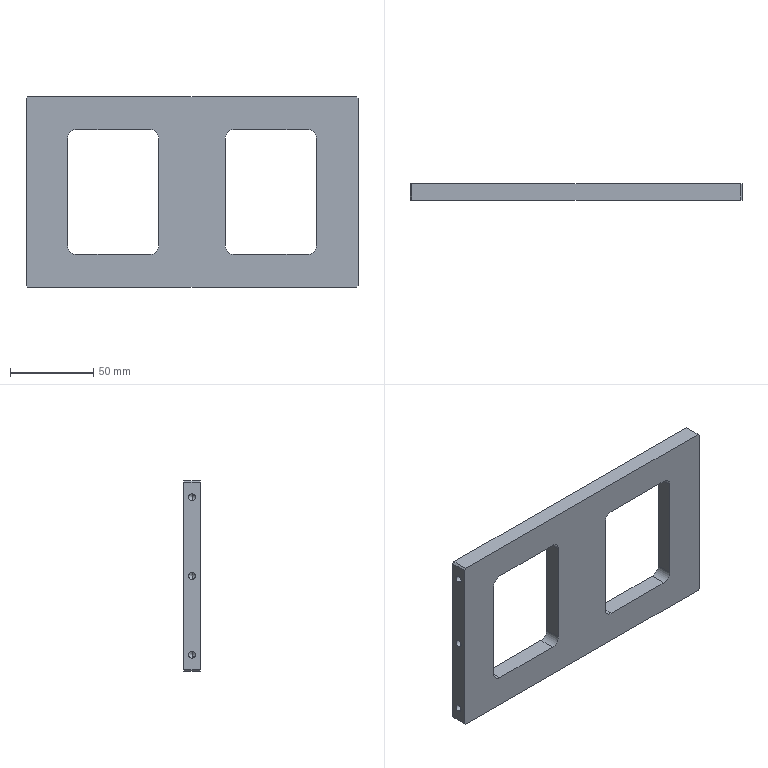Part | SolidWorks | features BaseBody 1 | 1 solid | 50 faces | box 200 x 10 x 115 mm | volume 146843 mm3 | cylinder 20 | plane 18 | cone 12 | commonest cylinder face diameters 4.2 x12 10 x8
STEP:
#1=CARTESIAN_POINT('',(87.6,0.,-45.4));
#2=VERTEX_POINT('',#1);
#3=CARTESIAN_POINT('',(100.,0.,-45.4));
#4=VERTEX_POINT('',#3);
#5=CARTESIAN_POINT('',(100.,0.,-45.4));
#6=DIRECTION('',(1.,0.,0.));
#7=VECTOR('',#6,1000.);
#8=LINE('',#5,#7);
#9=EDGE_CURVE('',#2,#4,#8,.T.);
#10=ORIENTED_EDGE('',*,*,#9,.F.);
#11=CARTESIAN_POINT('',(87.6,0.,-49.6));
#12=VERTEX_POINT('',#11);
#13=CARTESIAN_POINT('',(87.6,0.,-47.5));
#14=DIRECTION('',(1.,0.,0.));
#15=DIRECTION('',(0.,0.,-1.));
#16=AXIS2_PLACEMENT_3D('',#13,#14,#15);
#17=CIRCLE('',#16,2.1);
#18=EDGE_CURVE('',#12,#2,#17,.T.);
#19=ORIENTED_EDGE('',*,*,#18,.F.);
#20=CARTESIAN_POINT('',(100.,0.,-49.6));
#21=VERTEX_POINT('',#20);
#22=CARTESIAN_POINT('',(100.,0.,-49.6));
#23=DIRECTION('',(1.,0.,0.));
#24=VECTOR('',#23,1000.);
#25=LINE('',#22,#24);
#26=EDGE_CURVE('',#12,#21,#25,.T.);
#27=ORIENTED_EDGE('',*,*,#26,.T.);
#28=CARTESIAN_POINT('',(100.,0.,-47.5));
#29=DIRECTION('',(1.,0.,0.));
#30=DIRECTION('',(0.,0.,-1.));
#31=AXIS2_PLACEMENT_3D('',#28,#29,#30);
#32=CIRCLE('',#31,2.1);
#33=EDGE_CURVE('',#21,#4,#32,.T.);
#34=ORIENTED_EDGE('',*,*,#33,.T.);
#35=EDGE_LOOP('',(#10,#19,#27,#34));
#36=FACE_OUTER_BOUND('',#35,.T.);
#37=CARTESIAN_POINT('',(100.,0.,-47.5));
#38=DIRECTION('',(1.,0.,0.));
#39=DIRECTION('',(0.,0.,-1.));
#40=AXIS2_PLACEMENT_3D('',#37,#38,#39);
#41=CYLINDRICAL_SURFACE('',#40,2.1);
#42=ADVANCED_FACE('',(#36),#41,.F.);
#43=CARTESIAN_POINT('',(86.338,0.,-47.5));
#44=VERTEX_POINT('',#43);
#45=CARTESIAN_POINT('',(87.6,0.,-45.4));
#46=DIRECTION('',(0.515,0.,0.8572));
#47=VECTOR('',#46,1000.);
#48=LINE('',#45,#47);
#49=EDGE_CURVE('',#44,#2,#48,.T.);
#50=ORIENTED_EDGE('',*,*,#49,.F.);
#51=CARTESIAN_POINT('',(87.6,0.,-49.6));
#52=DIRECTION('',(0.515,0.,-0.8572));
#53=VECTOR('',#52,1000.);
#54=LINE('',#51,#53);
#55=EDGE_CURVE('',#44,#12,#54,.T.);
#56=ORIENTED_EDGE('',*,*,#55,.T.);
#57=ORIENTED_EDGE('',*,*,#18,.T.);
#58=EDGE_LOOP('',(#50,#56,#57));
#59=FACE_OUTER_BOUND('',#58,.T.);
#60=CARTESIAN_POINT('',(87.6,0.,-47.5));
#61=DIRECTION('',(1.,0.,0.));
#62=DIRECTION('',(0.,0.,-1.));
#63=AXIS2_PLACEMENT_3D('',#60,#61,#62);
#64=CONICAL_SURFACE('',#63,2.1,1.03);
#65=ADVANCED_FACE('',(#59),#64,.F.);
#66=CARTESIAN_POINT('',(87.6,0.,2.1));
#67=VERTEX_POINT('',#66);
#68=CARTESIAN_POINT('',(100.,0.,2.1));
#69=VERTEX_POINT('',#68);
#70=CARTESIAN_POINT('',(100.,0.,2.1));
#71=DIRECTION('',(1.,0.,0.));
#72=VECTOR('',#71,1000.);
#73=LINE('',#70,#72);
#74=EDGE_CURVE('',#67,#69,#73,.T.);
#75=ORIENTED_EDGE('',*,*,#74,.F.);
#76=CARTESIAN_POINT('',(87.6,0.,-2.1));
#77=VERTEX_POINT('',#76);
#78=CARTESIAN_POINT('',(87.6,0.,0.));
#79=DIRECTION('',(1.,0.,0.));
#80=DIRECTION('',(0.,0.,-1.));
#81=AXIS2_PLACEMENT_3D('',#78,#79,#80);
#82=CIRCLE('',#81,2.1);
#83=EDGE_CURVE('',#77,#67,#82,.T.);
#84=ORIENTED_EDGE('',*,*,#83,.F.);
#85=CARTESIAN_POINT('',(100.,0.,-2.1));
#86=VERTEX_POINT('',#85);
#87=CARTESIAN_POINT('',(100.,0.,-2.1));
#88=DIRECTION('',(1.,0.,0.));
#89=VECTOR('',#88,1000.);
#90=LINE('',#87,#89);
#91=EDGE_CURVE('',#77,#86,#90,.T.);
#92=ORIENTED_EDGE('',*,*,#91,.T.);
#93=CARTESIAN_POINT('',(100.,0.,0.));
#94=DIRECTION('',(1.,0.,0.));
#95=DIRECTION('',(0.,0.,-1.));
#96=AXIS2_PLACEMENT_3D('',#93,#94,#95);
#97=CIRCLE('',#96,2.1);
#98=EDGE_CURVE('',#86,#69,#97,.T.);
#99=ORIENTED_EDGE('',*,*,#98,.T.);
#100=EDGE_LOOP('',(#75,#84,#92,#99));
#101=FACE_OUTER_BOUND('',#100,.T.);
#102=CARTESIAN_POINT('',(100.,0.,0.));
#103=DIRECTION('',(1.,0.,0.));
#104=DIRECTION('',(0.,0.,-1.));
#105=AXIS2_PLACEMENT_3D('',#102,#103,#104);
#106=CYLINDRICAL_SURFACE('',#105,2.1);
#107=ADVANCED_FACE('',(#101),#106,.F.);
#108=CARTESIAN_POINT('',(86.338,0.,0.));
#109=VERTEX_POINT('',#108);
#110=CARTESIAN_POINT('',(87.6,0.,2.1));
#111=DIRECTION('',(0.515,0.,0.8572));
#112=VECTOR('',#111,1000.);
#113=LINE('',#110,#112);
#114=EDGE_CURVE('',#109,#67,#113,.T.);
#115=ORIENTED_EDGE('',*,*,#114,.F.);
#116=CARTESIAN_POINT('',(87.6,0.,-2.1));
#117=DIRECTION('',(0.515,0.,-0.8572));
#118=VECTOR('',#117,1000.);
#119=LINE('',#116,#118);
#120=EDGE_CURVE('',#109,#77,#119,.T.);
#121=ORIENTED_EDGE('',*,*,#120,.T.);
#122=ORIENTED_EDGE('',*,*,#83,.T.);
#123=EDGE_LOOP('',(#115,#121,#122));
#124=FACE_OUTER_BOUND('',#123,.T.);
#125=CARTESIAN_POINT('',(87.6,0.,0.));
#126=DIRECTION('',(1.,0.,0.));
#127=DIRECTION('',(0.,0.,-1.));
#128=AXIS2_PLACEMENT_3D('',#125,#126,#127);
#129=CONICAL_SURFACE('',#128,2.1,1.03);
#130=ADVANCED_FACE('',(#124),#129,.F.);
#131=CARTESIAN_POINT('',(87.6,0.,49.6));
#132=VERTEX_POINT('',#131);
#133=CARTESIAN_POINT('',(100.,0.,49.6));
#134=VERTEX_POINT('',#133);
#135=CARTESIAN_POINT('',(100.,0.,49.6));
#136=DIRECTION('',(1.,0.,0.));
#137=VECTOR('',#136,1000.);
#138=LINE('',#135,#137);
#139=EDGE_CURVE('',#132,#134,#138,.T.);
#140=ORIENTED_EDGE('',*,*,#139,.F.);
#141=CARTESIAN_POINT('',(87.6,0.,45.4));
#142=VERTEX_POINT('',#141);
#143=CARTESIAN_POINT('',(87.6,0.,47.5));
#144=DIRECTION('',(1.,0.,0.));
#145=DIRECTION('',(0.,0.,-1.));
#146=AXIS2_PLACEMENT_3D('',#143,#144,#145);
#147=CIRCLE('',#146,2.1);
#148=EDGE_CURVE('',#142,#132,#147,.T.);
#149=ORIENTED_EDGE('',*,*,#148,.F.);
#150=CARTESIAN_POINT('',(100.,0.,45.4));
#151=VERTEX_POINT('',#150);
#152=CARTESIAN_POINT('',(100.,0.,45.4));
#153=DIRECTION('',(1.,0.,0.));
#154=VECTOR('',#153,1000.);
#155=LINE('',#152,#154);
#156=EDGE_CURVE('',#142,#151,#155,.T.);
#157=ORIENTED_EDGE('',*,*,#156,.T.);
#158=CARTESIAN_POINT('',(100.,0.,47.5));
#159=DIRECTION('',(1.,0.,0.));
#160=DIRECTION('',(0.,0.,-1.));
#161=AXIS2_PLACEMENT_3D('',#158,#159,#160);
#162=CIRCLE('',#161,2.1);
#163=EDGE_CURVE('',#151,#134,#162,.T.);
#164=ORIENTED_EDGE('',*,*,#163,.T.);
#165=EDGE_LOOP('',(#140,#149,#157,#164));
#166=FACE_OUTER_BOUND('',#165,.T.);
#167=CARTESIAN_POINT('',(100.,0.,47.5));
#168=DIRECTION('',(1.,0.,0.));
#169=DIRECTION('',(0.,0.,-1.));
#170=AXIS2_PLACEMENT_3D('',#167,#168,#169);
#171=CYLINDRICAL_SURFACE('',#170,2.1);
#172=ADVANCED_FACE('',(#166),#171,.F.);
#173=CARTESIAN_POINT('',(86.338,0.,47.5));
#174=VERTEX_POINT('',#173);
#175=CARTESIAN_POINT('',(87.6,0.,49.6));
#176=DIRECTION('',(0.515,0.,0.8572));
#177=VECTOR('',#176,1000.);
#178=LINE('',#175,#177);
#179=EDGE_CURVE('',#174,#132,#178,.T.);
#180=ORIENTED_EDGE('',*,*,#179,.F.);
#181=CARTESIAN_POINT('',(87.6,0.,45.4));
#182=DIRECTION('',(0.515,0.,-0.8572));
#183=VECTOR('',#182,1000.);
#184=LINE('',#181,#183);
#185=EDGE_CURVE('',#174,#142,#184,.T.);
#186=ORIENTED_EDGE('',*,*,#185,.T.);
#187=ORIENTED_EDGE('',*,*,#148,.T.);
#188=EDGE_LOOP('',(#180,#186,#187));
#189=FACE_OUTER_BOUND('',#188,.T.);
#190=CARTESIAN_POINT('',(87.6,0.,47.5));
#191=DIRECTION('',(1.,0.,0.));
#192=DIRECTION('',(0.,0.,-1.));
#193=AXIS2_PLACEMENT_3D('',#190,#191,#192);
#194=CONICAL_SURFACE('',#193,2.1,1.03);
#195=ADVANCED_FACE('',(#189),#194,.F.);
#196=CARTESIAN_POINT('',(75.,-5.,-32.5));
#197=VERTEX_POINT('',#196);
#198=CARTESIAN_POINT('',(75.,5.,-32.5));
#199=VERTEX_POINT('',#198);
#200=CARTESIAN_POINT('',(75.,-98.005,-32.5));
#201=DIRECTION('',(0.,1.,0.));
#202=VECTOR('',#201,1000.);
#203=LINE('',#200,#202);
#204=EDGE_CURVE('',#197,#199,#203,.T.);
#205=ORIENTED_EDGE('',*,*,#204,.T.);
#206=CARTESIAN_POINT('',(70.,5.,-37.5));
#207=VERTEX_POINT('',#206);
#208=CARTESIAN_POINT('',(70.,5.,-32.5));
#209=DIRECTION('',(0.,1.,0.));
#210=DIRECTION('',(0.,0.,-1.));
#211=AXIS2_PLACEMENT_3D('',#208,#209,#210);
#212=CIRCLE('',#211,5.);
#213=EDGE_CURVE('',#199,#207,#212,.T.);
#214=ORIENTED_EDGE('',*,*,#213,.T.);
#215=CARTESIAN_POINT('',(70.,-5.,-37.5));
#216=VERTEX_POINT('',#215);
#217=CARTESIAN_POINT('',(70.,-98.005,-37.5));
#218=DIRECTION('',(0.,1.,0.));
#219=VECTOR('',#218,1000.);
#220=LINE('',#217,#219);
#221=EDGE_CURVE('',#216,#207,#220,.T.);
#222=ORIENTED_EDGE('',*,*,#221,.F.);
#223=CARTESIAN_POINT('',(70.,-5.,-32.5));
#224=DIRECTION('',(0.,1.,0.));
#225=DIRECTION('',(0.,0.,-1.));
#226=AXIS2_PLACEMENT_3D('',#223,#224,#225);
#227=CIRCLE('',#226,5.);
#228=EDGE_CURVE('',#197,#216,#227,.T.);
#229=ORIENTED_EDGE('',*,*,#228,.F.);
#230=EDGE_LOOP('',(#205,#214,#222,#229));
#231=FACE_OUTER_BOUND('',#230,.T.);
#232=CARTESIAN_POINT('',(70.,-98.005,-32.5));
#233=DIRECTION('',(0.,1.,0.));
#234=DIRECTION('',(0.,0.,1.));
#235=AXIS2_PLACEMENT_3D('',#232,#233,#234);
#236=CYLINDRICAL_SURFACE('',#235,5.);
#237=ADVANCED_FACE('',(#231),#236,.F.);
#238=CARTESIAN_POINT('',(75.,-5.,32.5));
#239=VERTEX_POINT('',#238);
#240=CARTESIAN_POINT('',(75.,5.,32.5));
#241=VERTEX_POINT('',#240);
#242=CARTESIAN_POINT('',(75.,-98.005,32.5));
#243=DIRECTION('',(0.,1.,0.));
#244=VECTOR('',#243,1000.);
#245=LINE('',#242,#244);
#246=EDGE_CURVE('',#239,#241,#245,.T.);
#247=ORIENTED_EDGE('',*,*,#246,.T.);
#248=CARTESIAN_POINT('',(75.,5.,-32.5));
#249=DIRECTION('',(0.,0.,-1.));
#250=VECTOR('',#249,1000.);
#251=LINE('',#248,#250);
#252=EDGE_CURVE('',#241,#199,#251,.T.);
#253=ORIENTED_EDGE('',*,*,#252,.T.);
#254=ORIENTED_EDGE('',*,*,#204,.F.);
#255=CARTESIAN_POINT('',(75.,-5.,-32.5));
#256=DIRECTION('',(0.,0.,-1.));
#257=VECTOR('',#256,1000.);
#258=LINE('',#255,#257);
#259=EDGE_CURVE('',#239,#197,#258,.T.);
#260=ORIENTED_EDGE('',*,*,#259,.F.);
#261=EDGE_LOOP('',(#247,#253,#254,#260));
#262=FACE_OUTER_BOUND('',#261,.T.);
#263=CARTESIAN_POINT('',(75.,-98.005,-32.5));
#264=DIRECTION('',(1.,0.,0.));
#265=DIRECTION('',(0.,1.,0.));
#266=AXIS2_PLACEMENT_3D('',#263,#264,#265);
#267=PLANE('',#266);
#268=ADVANCED_FACE('',(#262),#267,.F.);
#269=CARTESIAN_POINT('',(70.,-5.,37.5));
#270=VERTEX_POINT('',#269);
#271=CARTESIAN_POINT('',(70.,5.,37.5));
#272=VERTEX_POINT('',#271);
#273=CARTESIAN_POINT('',(70.,-98.005,37.5));
#274=DIRECTION('',(0.,1.,0.));
#275=VECTOR('',#274,1000.);
#276=LINE('',#273,#275);
#277=EDGE_CURVE('',#270,#272,#276,.T.);
#278=ORIENTED_EDGE('',*,*,#277,.T.);
#279=CARTESIAN_POINT('',(70.,5.,32.5));
#280=DIRECTION('',(0.,1.,0.));
#281=DIRECTION('',(0.,0.,1.));
#282=AXIS2_PLACEMENT_3D('',#279,#280,#281);
#283=CIRCLE('',#282,5.);
#284=EDGE_CURVE('',#272,#241,#283,.T.);
#285=ORIENTED_EDGE('',*,*,#284,.T.);
#286=ORIENTED_EDGE('',*,*,#246,.F.);
#287=CARTESIAN_POINT('',(70.,-5.,32.5));
#288=DIRECTION('',(0.,1.,0.));
#289=DIRECTION('',(0.,0.,-1.));
#290=AXIS2_PLACEMENT_3D('',#287,#288,#289);
#291=CIRCLE('',#290,5.);
#292=EDGE_CURVE('',#270,#239,#291,.T.);
#293=ORIENTED_EDGE('',*,*,#292,.F.);
#294=EDGE_LOOP('',(#278,#285,#286,#293));
#295=FACE_OUTER_BOUND('',#294,.T.);
#296=CARTESIAN_POINT('',(70.,-98.005,32.5));
#297=DIRECTION('',(0.,1.,0.));
#298=DIRECTION('',(0.,0.,1.));
#299=AXIS2_PLACEMENT_3D('',#296,#297,#298);
#300=CYLINDRICAL_SURFACE('',#299,5.);
#301=ADVANCED_FACE('',(#295),#300,.F.);
#302=CARTESIAN_POINT('',(25.,-5.,37.5));
#303=VERTEX_POINT('',#302);
#304=CARTESIAN_POINT('',(25.,5.,37.5));
#305=VERTEX_POINT('',#304);
#306=CARTESIAN_POINT('',(25.,-98.005,37.5));
#307=DIRECTION('',(0.,1.,0.));
#308=VECTOR('',#307,1000.);
#309=LINE('',#306,#308);
#310=EDGE_CURVE('',#303,#305,#309,.T.);
#311=ORIENTED_EDGE('',*,*,#310,.T.);
#312=CARTESIAN_POINT('',(25.,5.,37.5));
#313=DIRECTION('',(1.,0.,0.));
#314=VECTOR('',#313,1000.);
#315=LINE('',#312,#314);
#316=EDGE_CURVE('',#305,#272,#315,.T.);
#317=ORIENTED_EDGE('',*,*,#316,.T.);
#318=ORIENTED_EDGE('',*,*,#277,.F.);
#319=CARTESIAN_POINT('',(25.,-5.,37.5));
#320=DIRECTION('',(1.,0.,0.));
#321=VECTOR('',#320,1000.);
#322=LINE('',#319,#321);
#323=EDGE_CURVE('',#303,#270,#322,.T.);
#324=ORIENTED_EDGE('',*,*,#323,.F.);
#325=EDGE_LOOP('',(#311,#317,#318,#324));
#326=FACE_OUTER_BOUND('',#325,.T.);
#327=CARTESIAN_POINT('',(25.,-98.005,37.5));
#328=DIRECTION('',(0.,0.,1.));
#329=DIRECTION('',(1.,0.,0.));
#330=AXIS2_PLACEMENT_3D('',#327,#328,#329);
#331=PLANE('',#330);
#332=ADVANCED_FACE('',(#326),#331,.F.);
#333=CARTESIAN_POINT('',(20.,-5.,32.5));
#334=VERTEX_POINT('',#333);
#335=CARTESIAN_POINT('',(20.,5.,32.5));
#336=VERTEX_POINT('',#335);
#337=CARTESIAN_POINT('',(20.,-98.005,32.5));
#338=DIRECTION('',(0.,1.,0.));
#339=VECTOR('',#338,1000.);
#340=LINE('',#337,#339);
#341=EDGE_CURVE('',#334,#336,#340,.T.);
#342=ORIENTED_EDGE('',*,*,#341,.T.);
#343=CARTESIAN_POINT('',(25.,5.,32.5));
#344=DIRECTION('',(0.,1.,0.));
#345=DIRECTION('',(0.,0.,1.));
#346=AXIS2_PLACEMENT_3D('',#343,#344,#345);
#347=CIRCLE('',#346,5.);
#348=EDGE_CURVE('',#336,#305,#347,.T.);
#349=ORIENTED_EDGE('',*,*,#348,.T.);
#350=ORIENTED_EDGE('',*,*,#310,.F.);
#351=CARTESIAN_POINT('',(25.,-5.,32.5));
#352=DIRECTION('',(0.,1.,0.));
#353=DIRECTION('',(0.,0.,-1.));
#354=AXIS2_PLACEMENT_3D('',#351,#352,#353);
#355=CIRCLE('',#354,5.);
#356=EDGE_CURVE('',#334,#303,#355,.T.);
#357=ORIENTED_EDGE('',*,*,#356,.F.);
#358=EDGE_LOOP('',(#342,#349,#350,#357));
#359=FACE_OUTER_BOUND('',#358,.T.);
#360=CARTESIAN_POINT('',(25.,-98.005,32.5));
#361=DIRECTION('',(0.,1.,0.));
#362=DIRECTION('',(0.,0.,1.));
#363=AXIS2_PLACEMENT_3D('',#360,#361,#362);
#364=CYLINDRICAL_SURFACE('',#363,5.);
#365=ADVANCED_FACE('',(#359),#364,.F.);
#366=CARTESIAN_POINT('',(20.,-5.,-32.5));
#367=VERTEX_POINT('',#366);
#368=CARTESIAN_POINT('',(20.,5.,-32.5));
#369=VERTEX_POINT('',#368);
#370=CARTESIAN_POINT('',(20.,-98.005,-32.5));
#371=DIRECTION('',(0.,1.,0.));
#372=VECTOR('',#371,1000.);
#373=LINE('',#370,#372);
#374=EDGE_CURVE('',#367,#369,#373,.T.);
#375=ORIENTED_EDGE('',*,*,#374,.T.);
#376=CARTESIAN_POINT('',(20.,5.,-32.5));
#377=DIRECTION('',(0.,0.,1.));
#378=VECTOR('',#377,1000.);
#379=LINE('',#376,#378);
#380=EDGE_CURVE('',#369,#336,#379,.T.);
#381=ORIENTED_EDGE('',*,*,#380,.T.);
#382=ORIENTED_EDGE('',*,*,#341,.F.);
#383=CARTESIAN_POINT('',(20.,-5.,-32.5));
#384=DIRECTION('',(0.,0.,1.));
#385=VECTOR('',#384,1000.);
#386=LINE('',#383,#385);
#387=EDGE_CURVE('',#367,#334,#386,.T.);
#388=ORIENTED_EDGE('',*,*,#387,.F.);
#389=EDGE_LOOP('',(#375,#381,#382,#388));
#390=FACE_OUTER_BOUND('',#389,.T.);
#391=CARTESIAN_POINT('',(20.,-98.005,-32.5));
#392=DIRECTION('',(-1.,0.,0.));
#393=DIRECTION('',(0.,1.,0.));
#394=AXIS2_PLACEMENT_3D('',#391,#392,#393);
#395=PLANE('',#394);
#396=ADVANCED_FACE('',(#390),#395,.F.);
#397=CARTESIAN_POINT('',(25.,-5.,-37.5));
#398=VERTEX_POINT('',#397);
#399=CARTESIAN_POINT('',(25.,5.,-37.5));
#400=VERTEX_POINT('',#399);
#401=CARTESIAN_POINT('',(25.,-98.005,-37.5));
#402=DIRECTION('',(0.,1.,0.));
#403=VECTOR('',#402,1000.);
#404=LINE('',#401,#403);
#405=EDGE_CURVE('',#398,#400,#404,.T.);
#406=ORIENTED_EDGE('',*,*,#405,.T.);
#407=CARTESIAN_POINT('',(25.,5.,-32.5));
#408=DIRECTION('',(0.,1.,0.));
#409=DIRECTION('',(0.,0.,1.));
#410=AXIS2_PLACEMENT_3D('',#407,#408,#409);
#411=CIRCLE('',#410,5.);
#412=EDGE_CURVE('',#400,#369,#411,.T.);
#413=ORIENTED_EDGE('',*,*,#412,.T.);
#414=ORIENTED_EDGE('',*,*,#374,.F.);
#415=CARTESIAN_POINT('',(25.,-5.,-32.5));
#416=DIRECTION('',(0.,1.,0.));
#417=DIRECTION('',(0.,0.,-1.));
#418=AXIS2_PLACEMENT_3D('',#415,#416,#417);
#419=CIRCLE('',#418,5.);
#420=EDGE_CURVE('',#398,#367,#419,.T.);
#421=ORIENTED_EDGE('',*,*,#420,.F.);
#422=EDGE_LOOP('',(#406,#413,#414,#421));
#423=FACE_OUTER_BOUND('',#422,.T.);
#424=CARTESIAN_POINT('',(25.,-98.005,-32.5));
#425=DIRECTION('',(0.,1.,0.));
#426=DIRECTION('',(0.,0.,1.));
#427=AXIS2_PLACEMENT_3D('',#424,#425,#426);
#428=CYLINDRICAL_SURFACE('',#427,5.);
#429=ADVANCED_FACE('',(#423),#428,.F.);
#430=ORIENTED_EDGE('',*,*,#221,.T.);
#431=CARTESIAN_POINT('',(25.,5.,-37.5));
#432=DIRECTION('',(-1.,0.,0.));
#433=VECTOR('',#432,1000.);
#434=LINE('',#431,#433);
#435=EDGE_CURVE('',#207,#400,#434,.T.);
#436=ORIENTED_EDGE('',*,*,#435,.T.);
#437=ORIENTED_EDGE('',*,*,#405,.F.);
#438=CARTESIAN_POINT('',(25.,-5.,-37.5));
#439=DIRECTION('',(-1.,0.,0.));
#440=VECTOR('',#439,1000.);
#441=LINE('',#438,#440);
#442=EDGE_CURVE('',#216,#398,#441,.T.);
#443=ORIENTED_EDGE('',*,*,#442,.F.);
#444=EDGE_LOOP('',(#430,#436,#437,#443));
#445=FACE_OUTER_BOUND('',#444,.T.);
#446=CARTESIAN_POINT('',(25.,-98.005,-37.5));
#447=DIRECTION('',(0.,0.,-1.));
#448=DIRECTION('',(-1.,0.,0.));
#449=AXIS2_PLACEMENT_3D('',#446,#447,#448);
#450=PLANE('',#449);
#451=ADVANCED_FACE('',(#445),#450,.F.);
#452=CARTESIAN_POINT('',(-20.,-5.,-32.5));
#453=VERTEX_POINT('',#452);
#454=CARTESIAN_POINT('',(-20.,5.,-32.5));
#455=VERTEX_POINT('',#454);
#456=CARTESIAN_POINT('',(-20.,-98.005,-32.5));
#457=DIRECTION('',(0.,1.,0.));
#458=VECTOR('',#457,1000.);
#459=LINE('',#456,#458);
#460=EDGE_CURVE('',#453,#455,#459,.T.);
#461=ORIENTED_EDGE('',*,*,#460,.T.);
#462=CARTESIAN_POINT('',(-25.,5.,-37.5));
#463=VERTEX_POINT('',#462);
#464=CARTESIAN_POINT('',(-25.,5.,-32.5));
#465=DIRECTION('',(0.,1.,0.));
#466=DIRECTION('',(0.,0.,-1.));
#467=AXIS2_PLACEMENT_3D('',#464,#465,#466);
#468=CIRCLE('',#467,5.);
#469=EDGE_CURVE('',#455,#463,#468,.T.);
#470=ORIENTED_EDGE('',*,*,#469,.T.);
#471=CARTESIAN_POINT('',(-25.,-5.,-37.5));
#472=VERTEX_POINT('',#471);
#473=CARTESIAN_POINT('',(-25.,-98.005,-37.5));
#474=DIRECTION('',(0.,1.,0.));
#475=VECTOR('',#474,1000.);
#476=LINE('',#473,#475);
#477=EDGE_CURVE('',#472,#463,#476,.T.);
#478=ORIENTED_EDGE('',*,*,#477,.F.);
#479=CARTESIAN_POINT('',(-25.,-5.,-32.5));
#480=DIRECTION('',(0.,1.,0.));
#481=DIRECTION('',(0.,0.,-1.));
#482=AXIS2_PLACEMENT_3D('',#479,#480,#481);
#483=CIRCLE('',#482,5.);
#484=EDGE_CURVE('',#453,#472,#483,.T.);
#485=ORIENTED_EDGE('',*,*,#484,.F.);
#486=EDGE_LOOP('',(#461,#470,#478,#485));
#487=FACE_OUTER_BOUND('',#486,.T.);
#488=CARTESIAN_POINT('',(-25.,-98.005,-32.5));
#489=DIRECTION('',(0.,1.,0.));
#490=DIRECTION('',(0.,0.,1.));
#491=AXIS2_PLACEMENT_3D('',#488,#489,#490);
#492=CYLINDRICAL_SURFACE('',#491,5.);
#493=ADVANCED_FACE('',(#487),#492,.F.);
#494=CARTESIAN_POINT('',(-20.,-5.,32.5));
#495=VERTEX_POINT('',#494);
#496=CARTESIAN_POINT('',(-20.,5.,32.5));
#497=VERTEX_POINT('',#496);
#498=CARTESIAN_POINT('',(-20.,-98.005,32.5));
#499=DIRECTION('',(0.,1.,0.));
#500=VECTOR('',#499,1000.);
#501=LINE('',#498,#500);
#502=EDGE_CURVE('',#495,#497,#501,.T.);
#503=ORIENTED_EDGE('',*,*,#502,.T.);
#504=CARTESIAN_POINT('',(-20.,5.,-32.5));
#505=DIRECTION('',(0.,0.,-1.));
#506=VECTOR('',#505,1000.);
#507=LINE('',#504,#506);
#508=EDGE_CURVE('',#497,#455,#507,.T.);
#509=ORIENTED_EDGE('',*,*,#508,.T.);
#510=ORIENTED_EDGE('',*,*,#460,.F.);
#511=CARTESIAN_POINT('',(-20.,-5.,-32.5));
#512=DIRECTION('',(0.,0.,-1.));
#513=VECTOR('',#512,1000.);
#514=LINE('',#511,#513);
#515=EDGE_CURVE('',#495,#453,#514,.T.);
#516=ORIENTED_EDGE('',*,*,#515,.F.);
#517=EDGE_LOOP('',(#503,#509,#510,#516));
#518=FACE_OUTER_BOUND('',#517,.T.);
#519=CARTESIAN_POINT('',(-20.,-98.005,-32.5));
#520=DIRECTION('',(1.,0.,0.));
#521=DIRECTION('',(0.,0.,1.));
#522=AXIS2_PLACEMENT_3D('',#519,#520,#521);
#523=PLANE('',#522);
#524=ADVANCED_FACE('',(#518),#523,.F.);
#525=CARTESIAN_POINT('',(-25.,-5.,37.5));
#526=VERTEX_POINT('',#525);
#527=CARTESIAN_POINT('',(-25.,5.,37.5));
#528=VERTEX_POINT('',#527);
#529=CARTESIAN_POINT('',(-25.,-98.005,37.5));
#530=DIRECTION('',(0.,1.,0.));
#531=VECTOR('',#530,1000.);
#532=LINE('',#529,#531);
#533=EDGE_CURVE('',#526,#528,#532,.T.);
#534=ORIENTED_EDGE('',*,*,#533,.T.);
#535=CARTESIAN_POINT('',(-25.,5.,32.5));
#536=DIRECTION('',(0.,1.,0.));
#537=DIRECTION('',(0.,0.,-1.));
#538=AXIS2_PLACEMENT_3D('',#535,#536,#537);
#539=CIRCLE('',#538,5.);
#540=EDGE_CURVE('',#528,#497,#539,.T.);
#541=ORIENTED_EDGE('',*,*,#540,.T.);
#542=ORIENTED_EDGE('',*,*,#502,.F.);
#543=CARTESIAN_POINT('',(-25.,-5.,32.5));
#544=DIRECTION('',(0.,1.,0.));
#545=DIRECTION('',(0.,0.,-1.));
#546=AXIS2_PLACEMENT_3D('',#543,#544,#545);
#547=CIRCLE('',#546,5.);
#548=EDGE_CURVE('',#526,#495,#547,.T.);
#549=ORIENTED_EDGE('',*,*,#548,.F.);
#550=EDGE_LOOP('',(#534,#541,#542,#549));
#551=FACE_OUTER_BOUND('',#550,.T.);
#552=CARTESIAN_POINT('',(-25.,-98.005,32.5));
#553=DIRECTION('',(0.,1.,0.));
#554=DIRECTION('',(0.,0.,1.));
#555=AXIS2_PLACEMENT_3D('',#552,#553,#554);
#556=CYLINDRICAL_SURFACE('',#555,5.);
#557=ADVANCED_FACE('',(#551),#556,.F.);
#558=CARTESIAN_POINT('',(-70.,-5.,37.5));
#559=VERTEX_POINT('',#558);
#560=CARTESIAN_POINT('',(-70.,5.,37.5));
#561=VERTEX_POINT('',#560);
#562=CARTESIAN_POINT('',(-70.,-98.005,37.5));
#563=DIRECTION('',(0.,1.,0.));
#564=VECTOR('',#563,1000.);
#565=LINE('',#562,#564);
#566=EDGE_CURVE('',#559,#561,#565,.T.);
#567=ORIENTED_EDGE('',*,*,#566,.T.);
#568=CARTESIAN_POINT('',(-25.,5.,37.5));
#569=DIRECTION('',(1.,0.,0.));
#570=VECTOR('',#569,1000.);
#571=LINE('',#568,#570);
#572=EDGE_CURVE('',#561,#528,#571,.T.);
#573=ORIENTED_EDGE('',*,*,#572,.T.);
#574=ORIENTED_EDGE('',*,*,#533,.F.);
#575=CARTESIAN_POINT('',(-25.,-5.,37.5));
#576=DIRECTION('',(1.,0.,0.));
#577=VECTOR('',#576,1000.);
#578=LINE('',#575,#577);
#579=EDGE_CURVE('',#559,#526,#578,.T.);
#580=ORIENTED_EDGE('',*,*,#579,.F.);
#581=EDGE_LOOP('',(#567,#573,#574,#580));
#582=FACE_OUTER_BOUND('',#581,.T.);
#583=CARTESIAN_POINT('',(-25.,-98.005,37.5));
#584=DIRECTION('',(0.,0.,1.));
#585=DIRECTION('',(1.,0.,0.));
#586=AXIS2_PLACEMENT_3D('',#583,#584,#585);
#587=PLANE('',#586);
#588=ADVANCED_FACE('',(#582),#587,.F.);
#589=CARTESIAN_POINT('',(-75.,-5.,32.5));
#590=VERTEX_POINT('',#589);
#591=CARTESIAN_POINT('',(-75.,5.,32.5));
#592=VERTEX_POINT('',#591);
#593=CARTESIAN_POINT('',(-75.,-98.005,32.5));
#594=DIRECTION('',(0.,1.,0.));
#595=VECTOR('',#594,1000.);
#596=LINE('',#593,#595);
#597=EDGE_CURVE('',#590,#592,#596,.T.);
#598=ORIENTED_EDGE('',*,*,#597,.T.);
#599=CARTESIAN_POINT('',(-70.,5.,32.5));
#600=DIRECTION('',(0.,1.,0.));
#601=DIRECTION('',(0.,0.,-1.));
#602=AXIS2_PLACEMENT_3D('',#599,#600,#601);
#603=CIRCLE('',#602,5.);
#604=EDGE_CURVE('',#592,#561,#603,.T.);
#605=ORIENTED_EDGE('',*,*,#604,.T.);
#606=ORIENTED_EDGE('',*,*,#566,.F.);
#607=CARTESIAN_POINT('',(-70.,-5.,32.5));
#608=DIRECTION('',(0.,1.,0.));
#609=DIRECTION('',(0.,0.,-1.));
#610=AXIS2_PLACEMENT_3D('',#607,#608,#609);
#611=CIRCLE('',#610,5.);
#612=EDGE_CURVE('',#590,#559,#611,.T.);
#613=ORIENTED_EDGE('',*,*,#612,.F.);
#614=EDGE_LOOP('',(#598,#605,#606,#613));
#615=FACE_OUTER_BOUND('',#614,.T.);
#616=CARTESIAN_POINT('',(-70.,-98.005,32.5));
#617=DIRECTION('',(0.,1.,0.));
#618=DIRECTION('',(0.,0.,1.));
#619=AXIS2_PLACEMENT_3D('',#616,#617,#618);
#620=CYLINDRICAL_SURFACE('',#619,5.);
#621=ADVANCED_FACE('',(#615),#620,.F.);
#622=CARTESIAN_POINT('',(-75.,-5.,-32.5));
#623=VERTEX_POINT('',#622);
#624=CARTESIAN_POINT('',(-75.,5.,-32.5));
#625=VERTEX_POINT('',#624);
#626=CARTESIAN_POINT('',(-75.,-98.005,-32.5));
#627=DIRECTION('',(0.,1.,0.));
#628=VECTOR('',#627,1000.);
#629=LINE('',#626,#628);
#630=EDGE_CURVE('',#623,#625,#629,.T.);
#631=ORIENTED_EDGE('',*,*,#630,.T.);
#632=CARTESIAN_POINT('',(-75.,5.,-32.5));
#633=DIRECTION('',(0.,0.,1.));
#634=VECTOR('',#633,1000.);
#635=LINE('',#632,#634);
#636=EDGE_CURVE('',#625,#592,#635,.T.);
#637=ORIENTED_EDGE('',*,*,#636,.T.);
#638=ORIENTED_EDGE('',*,*,#597,.F.);
#639=CARTESIAN_POINT('',(-75.,-5.,-32.5));
#640=DIRECTION('',(0.,0.,1.));
#641=VECTOR('',#640,1000.);
#642=LINE('',#639,#641);
#643=EDGE_CURVE('',#623,#590,#642,.T.);
#644=ORIENTED_EDGE('',*,*,#643,.F.);
#645=EDGE_LOOP('',(#631,#637,#638,#644));
#646=FACE_OUTER_BOUND('',#645,.T.);
#647=CARTESIAN_POINT('',(-75.,-98.005,-32.5));
#648=DIRECTION('',(-1.,0.,0.));
#649=DIRECTION('',(0.,0.,1.));
#650=AXIS2_PLACEMENT_3D('',#647,#648,#649);
#651=PLANE('',#650);
#652=ADVANCED_FACE('',(#646),#651,.F.);
#653=CARTESIAN_POINT('',(-70.,-5.,-37.5));
#654=VERTEX_POINT('',#653);
#655=CARTESIAN_POINT('',(-70.,5.,-37.5));
#656=VERTEX_POINT('',#655);
#657=CARTESIAN_POINT('',(-70.,-98.005,-37.5));
#658=DIRECTION('',(0.,1.,0.));
#659=VECTOR('',#658,1000.);
#660=LINE('',#657,#659);
#661=EDGE_CURVE('',#654,#656,#660,.T.);
#662=ORIENTED_EDGE('',*,*,#661,.T.);
#663=CARTESIAN_POINT('',(-70.,5.,-32.5));
#664=DIRECTION('',(0.,1.,0.));
#665=DIRECTION('',(0.,0.,1.));
#666=AXIS2_PLACEMENT_3D('',#663,#664,#665);
#667=CIRCLE('',#666,5.);
#668=EDGE_CURVE('',#656,#625,#667,.T.);
#669=ORIENTED_EDGE('',*,*,#668,.T.);
#670=ORIENTED_EDGE('',*,*,#630,.F.);
#671=CARTESIAN_POINT('',(-70.,-5.,-32.5));
#672=DIRECTION('',(0.,1.,0.));
#673=DIRECTION('',(0.,0.,-1.));
#674=AXIS2_PLACEMENT_3D('',#671,#672,#673);
#675=CIRCLE('',#674,5.);
#676=EDGE_CURVE('',#654,#623,#675,.T.);
#677=ORIENTED_EDGE('',*,*,#676,.F.);
#678=EDGE_LOOP('',(#662,#669,#670,#677));
#679=FACE_OUTER_BOUND('',#678,.T.);
#680=CARTESIAN_POINT('',(-70.,-98.005,-32.5));
#681=DIRECTION('',(0.,1.,0.));
#682=DIRECTION('',(0.,0.,1.));
#683=AXIS2_PLACEMENT_3D('',#680,#681,#682);
#684=CYLINDRICAL_SURFACE('',#683,5.);
#685=ADVANCED_FACE('',(#679),#684,.F.);
#686=ORIENTED_EDGE('',*,*,#477,.T.);
#687=CARTESIAN_POINT('',(-25.,5.,-37.5));
#688=DIRECTION('',(-1.,0.,0.));
#689=VECTOR('',#688,1000.);
#690=LINE('',#687,#689);
#691=EDGE_CURVE('',#463,#656,#690,.T.);
#692=ORIENTED_EDGE('',*,*,#691,.T.);
#693=ORIENTED_EDGE('',*,*,#661,.F.);
#694=CARTESIAN_POINT('',(-25.,-5.,-37.5));
#695=DIRECTION('',(-1.,0.,0.));
#696=VECTOR('',#695,1000.);
#697=LINE('',#694,#696);
#698=EDGE_CURVE('',#472,#654,#697,.T.);
#699=ORIENTED_EDGE('',*,*,#698,.F.);
#700=EDGE_LOOP('',(#686,#692,#693,#699));
#701=FACE_OUTER_BOUND('',#700,.T.);
#702=CARTESIAN_POINT('',(-25.,-98.005,-37.5));
#703=DIRECTION('',(0.,0.,-1.));
#704=DIRECTION('',(0.,-1.,0.));
#705=AXIS2_PLACEMENT_3D('',#702,#703,#704);
#706=PLANE('',#705);
#707=ADVANCED_FACE('',(#701),#706,.F.);
#708=CARTESIAN_POINT('',(-87.6,0.,-49.6));
#709=VERTEX_POINT('',#708);
#710=CARTESIAN_POINT('',(-100.,0.,-49.6));
#711=VERTEX_POINT('',#710);
#712=CARTESIAN_POINT('',(-100.,0.,-49.6));
#713=DIRECTION('',(-1.,0.,0.));
#714=VECTOR('',#713,1000.);
#715=LINE('',#712,#714);
#716=EDGE_CURVE('',#709,#711,#715,.T.);
#717=ORIENTED_EDGE('',*,*,#716,.F.);
#718=CARTESIAN_POINT('',(-87.6,0.,-45.4));
#719=VERTEX_POINT('',#718);
#720=CARTESIAN_POINT('',(-87.6,0.,-47.5));
#721=DIRECTION('',(-1.,0.,0.));
#722=DIRECTION('',(0.,0.,1.));
#723=AXIS2_PLACEMENT_3D('',#720,#721,#722);
#724=CIRCLE('',#723,2.1);
#725=EDGE_CURVE('',#719,#709,#724,.T.);
#726=ORIENTED_EDGE('',*,*,#725,.F.);
#727=CARTESIAN_POINT('',(-100.,0.,-45.4));
#728=VERTEX_POINT('',#727);
#729=CARTESIAN_POINT('',(-100.,0.,-45.4));
#730=DIRECTION('',(-1.,0.,0.));
#731=VECTOR('',#730,1000.);
#732=LINE('',#729,#731);
#733=EDGE_CURVE('',#719,#728,#732,.T.);
#734=ORIENTED_EDGE('',*,*,#733,.T.);
#735=CARTESIAN_POINT('',(-100.,0.,-47.5));
#736=DIRECTION('',(-1.,0.,0.));
#737=DIRECTION('',(0.,0.,1.));
#738=AXIS2_PLACEMENT_3D('',#735,#736,#737);
#739=CIRCLE('',#738,2.1);
#740=EDGE_CURVE('',#728,#711,#739,.T.);
#741=ORIENTED_EDGE('',*,*,#740,.T.);
#742=EDGE_LOOP('',(#717,#726,#734,#741));
#743=FACE_OUTER_BOUND('',#742,.T.);
#744=CARTESIAN_POINT('',(-100.,0.,-47.5));
#745=DIRECTION('',(-1.,0.,0.));
#746=DIRECTION('',(0.,0.,1.));
#747=AXIS2_PLACEMENT_3D('',#744,#745,#746);
#748=CYLINDRICAL_SURFACE('',#747,2.1);
#749=ADVANCED_FACE('',(#743),#748,.F.);
#750=CARTESIAN_POINT('',(-86.338,0.,-47.5));
#751=VERTEX_POINT('',#750);
#752=CARTESIAN_POINT('',(-87.6,0.,-49.6));
#753=DIRECTION('',(-0.515,0.,-0.8572));
#754=VECTOR('',#753,1000.);
#755=LINE('',#752,#754);
#756=EDGE_CURVE('',#751,#709,#755,.T.);
#757=ORIENTED_EDGE('',*,*,#756,.F.);
#758=CARTESIAN_POINT('',(-87.6,0.,-45.4));
#759=DIRECTION('',(-0.515,0.,0.8572));
#760=VECTOR('',#759,1000.);
#761=LINE('',#758,#760);
#762=EDGE_CURVE('',#751,#719,#761,.T.);
#763=ORIENTED_EDGE('',*,*,#762,.T.);
#764=ORIENTED_EDGE('',*,*,#725,.T.);
#765=EDGE_LOOP('',(#757,#763,#764));
#766=FACE_OUTER_BOUND('',#765,.T.);
#767=CARTESIAN_POINT('',(-87.6,0.,-47.5));
#768=DIRECTION('',(-1.,0.,0.));
#769=DIRECTION('',(0.,0.,1.));
#770=AXIS2_PLACEMENT_3D('',#767,#768,#769);
#771=CONICAL_SURFACE('',#770,2.1,1.03);
#772=ADVANCED_FACE('',(#766),#771,.F.);
#773=CARTESIAN_POINT('',(-87.6,0.,-2.1));
#774=VERTEX_POINT('',#773);
#775=CARTESIAN_POINT('',(-100.,0.,-2.1));
#776=VERTEX_POINT('',#775);
#777=CARTESIAN_POINT('',(-100.,0.,-2.1));
#778=DIRECTION('',(-1.,0.,0.));
#779=VECTOR('',#778,1000.);
#780=LINE('',#777,#779);
#781=EDGE_CURVE('',#774,#776,#780,.T.);
#782=ORIENTED_EDGE('',*,*,#781,.F.);
#783=CARTESIAN_POINT('',(-87.6,0.,2.1));
#784=VERTEX_POINT('',#783);
#785=CARTESIAN_POINT('',(-87.6,0.,0.));
#786=DIRECTION('',(-1.,0.,0.));
#787=DIRECTION('',(0.,0.,1.));
#788=AXIS2_PLACEMENT_3D('',#785,#786,#787);
#789=CIRCLE('',#788,2.1);
#790=EDGE_CURVE('',#784,#774,#789,.T.);
#791=ORIENTED_EDGE('',*,*,#790,.F.);
#792=CARTESIAN_POINT('',(-100.,0.,2.1));
#793=VERTEX_POINT('',#792);
#794=CARTESIAN_POINT('',(-100.,0.,2.1));
#795=DIRECTION('',(-1.,0.,0.));
#796=VECTOR('',#795,1000.);
#797=LINE('',#794,#796);
#798=EDGE_CURVE('',#784,#793,#797,.T.);
#799=ORIENTED_EDGE('',*,*,#798,.T.);
#800=CARTESIAN_POINT('',(-100.,0.,0.));
#801=DIRECTION('',(-1.,0.,0.));
#802=DIRECTION('',(0.,0.,1.));
#803=AXIS2_PLACEMENT_3D('',#800,#801,#802);
#804=CIRCLE('',#803,2.1);
#805=EDGE_CURVE('',#793,#776,#804,.T.);
#806=ORIENTED_EDGE('',*,*,#805,.T.);
#807=EDGE_LOOP('',(#782,#791,#799,#806));
#808=FACE_OUTER_BOUND('',#807,.T.);
#809=CARTESIAN_POINT('',(-100.,0.,0.));
#810=DIRECTION('',(-1.,0.,0.));
#811=DIRECTION('',(0.,0.,1.));
#812=AXIS2_PLACEMENT_3D('',#809,#810,#811);
#813=CYLINDRICAL_SURFACE('',#812,2.1);
#814=ADVANCED_FACE('',(#808),#813,.F.);
#815=CARTESIAN_POINT('',(-86.338,0.,0.));
#816=VERTEX_POINT('',#815);
#817=CARTESIAN_POINT('',(-87.6,0.,-2.1));
#818=DIRECTION('',(-0.515,0.,-0.8572));
#819=VECTOR('',#818,1000.);
#820=LINE('',#817,#819);
#821=EDGE_CURVE('',#816,#774,#820,.T.);
#822=ORIENTED_EDGE('',*,*,#821,.F.);
#823=CARTESIAN_POINT('',(-87.6,0.,2.1));
#824=DIRECTION('',(-0.515,0.,0.8572));
#825=VECTOR('',#824,1000.);
#826=LINE('',#823,#825);
#827=EDGE_CURVE('',#816,#784,#826,.T.);
#828=ORIENTED_EDGE('',*,*,#827,.T.);
#829=ORIENTED_EDGE('',*,*,#790,.T.);
#830=EDGE_LOOP('',(#822,#828,#829));
#831=FACE_OUTER_BOUND('',#830,.T.);
#832=CARTESIAN_POINT('',(-87.6,0.,0.));
#833=DIRECTION('',(-1.,0.,0.));
#834=DIRECTION('',(0.,0.,1.));
#835=AXIS2_PLACEMENT_3D('',#832,#833,#834);
#836=CONICAL_SURFACE('',#835,2.1,1.03);
#837=ADVANCED_FACE('',(#831),#836,.F.);
#838=CARTESIAN_POINT('',(-87.6,0.,45.4));
#839=VERTEX_POINT('',#838);
#840=CARTESIAN_POINT('',(-100.,0.,45.4));
#841=VERTEX_POINT('',#840);
#842=CARTESIAN_POINT('',(-100.,0.,45.4));
#843=DIRECTION('',(-1.,0.,0.));
#844=VECTOR('',#843,1000.);
#845=LINE('',#842,#844);
#846=EDGE_CURVE('',#839,#841,#845,.T.);
#847=ORIENTED_EDGE('',*,*,#846,.F.);
#848=CARTESIAN_POINT('',(-87.6,0.,49.6));
#849=VERTEX_POINT('',#848);
#850=CARTESIAN_POINT('',(-87.6,0.,47.5));
#851=DIRECTION('',(-1.,0.,0.));
#852=DIRECTION('',(0.,0.,1.));
#853=AXIS2_PLACEMENT_3D('',#850,#851,#852);
#854=CIRCLE('',#853,2.1);
#855=EDGE_CURVE('',#849,#839,#854,.T.);
#856=ORIENTED_EDGE('',*,*,#855,.F.);
#857=CARTESIAN_POINT('',(-100.,0.,49.6));
#858=VERTEX_POINT('',#857);
#859=CARTESIAN_POINT('',(-100.,0.,49.6));
#860=DIRECTION('',(-1.,0.,0.));
#861=VECTOR('',#860,1000.);
#862=LINE('',#859,#861);
#863=EDGE_CURVE('',#849,#858,#862,.T.);
#864=ORIENTED_EDGE('',*,*,#863,.T.);
#865=CARTESIAN_POINT('',(-100.,0.,47.5));
#866=DIRECTION('',(-1.,0.,0.));
#867=DIRECTION('',(0.,0.,1.));
#868=AXIS2_PLACEMENT_3D('',#865,#866,#867);
#869=CIRCLE('',#868,2.1);
#870=EDGE_CURVE('',#858,#841,#869,.T.);
#871=ORIENTED_EDGE('',*,*,#870,.T.);
#872=EDGE_LOOP('',(#847,#856,#864,#871));
#873=FACE_OUTER_BOUND('',#872,.T.);
#874=CARTESIAN_POINT('',(-100.,0.,47.5));
#875=DIRECTION('',(-1.,0.,0.));
#876=DIRECTION('',(0.,0.,1.));
#877=AXIS2_PLACEMENT_3D('',#874,#875,#876);
#878=CYLINDRICAL_SURFACE('',#877,2.1);
#879=ADVANCED_FACE('',(#873),#878,.F.);
#880=CARTESIAN_POINT('',(-86.338,0.,47.5));
#881=VERTEX_POINT('',#880);
#882=CARTESIAN_POINT('',(-87.6,0.,45.4));
#883=DIRECTION('',(-0.515,0.,-0.8572));
#884=VECTOR('',#883,1000.);
#885=LINE('',#882,#884);
#886=EDGE_CURVE('',#881,#839,#885,.T.);
#887=ORIENTED_EDGE('',*,*,#886,.F.);
#888=CARTESIAN_POINT('',(-87.6,0.,49.6));
#889=DIRECTION('',(-0.515,0.,0.8572));
#890=VECTOR('',#889,1000.);
#891=LINE('',#888,#890);
#892=EDGE_CURVE('',#881,#849,#891,.T.);
#893=ORIENTED_EDGE('',*,*,#892,.T.);
#894=ORIENTED_EDGE('',*,*,#855,.T.);
#895=EDGE_LOOP('',(#887,#893,#894));
#896=FACE_OUTER_BOUND('',#895,.T.);
#897=CARTESIAN_POINT('',(-87.6,0.,47.5));
#898=DIRECTION('',(-1.,0.,0.));
#899=DIRECTION('',(0.,0.,1.));
#900=AXIS2_PLACEMENT_3D('',#897,#898,#899);
#901=CONICAL_SURFACE('',#900,2.1,1.03);
#902=ADVANCED_FACE('',(#896),#901,.F.);
#903=CARTESIAN_POINT('',(-100.,5.,56.5));
#904=VERTEX_POINT('',#903);
#905=CARTESIAN_POINT('',(-99.,5.,57.5));
#906=VERTEX_POINT('',#905);
#907=CARTESIAN_POINT('',(-99.,5.,57.5));
#908=DIRECTION('',(0.7071,0.,0.7071));
#909=VECTOR('',#908,1000.);
#910=LINE('',#907,#909);
#911=EDGE_CURVE('',#904,#906,#910,.T.);
#912=ORIENTED_EDGE('',*,*,#911,.F.);
#913=CARTESIAN_POINT('',(-100.,-5.,56.5));
#914=VERTEX_POINT('',#913);
#915=CARTESIAN_POINT('',(-100.,5.,56.5));
#916=DIRECTION('',(0.,1.,0.));
#917=VECTOR('',#916,1000.);
#918=LINE('',#915,#917);
#919=EDGE_CURVE('',#914,#904,#918,.T.);
#920=ORIENTED_EDGE('',*,*,#919,.F.);
#921=CARTESIAN_POINT('',(-99.,-5.,57.5));
#922=VERTEX_POINT('',#921);
#923=CARTESIAN_POINT('',(-78.25,-5.,78.25));
#924=DIRECTION('',(-0.7071,0.,-0.7071));
#925=VECTOR('',#924,1000.);
#926=LINE('',#923,#925);
#927=EDGE_CURVE('',#922,#914,#926,.T.);
#928=ORIENTED_EDGE('',*,*,#927,.F.);
#929=CARTESIAN_POINT('',(-99.,5.,57.5));
#930=DIRECTION('',(0.,-1.,0.));
#931=VECTOR('',#930,1000.);
#932=LINE('',#929,#931);
#933=EDGE_CURVE('',#906,#922,#932,.T.);
#934=ORIENTED_EDGE('',*,*,#933,.F.);
#935=EDGE_LOOP('',(#912,#920,#928,#934));
#936=FACE_OUTER_BOUND('',#935,.T.);
#937=CARTESIAN_POINT('',(-99.,5.,57.5));
#938=DIRECTION('',(0.7071,0.,-0.7071));
#939=DIRECTION('',(0.,-1.,0.));
#940=AXIS2_PLACEMENT_3D('',#937,#938,#939);
#941=PLANE('',#940);
#942=ADVANCED_FACE('',(#936),#941,.F.);
#943=CARTESIAN_POINT('',(-99.,5.,-57.5));
#944=VERTEX_POINT('',#943);
#945=CARTESIAN_POINT('',(-100.,5.,-56.5));
#946=VERTEX_POINT('',#945);
#947=CARTESIAN_POINT('',(-100.,5.,-56.5));
#948=DIRECTION('',(-0.7071,0.,0.7071));
#949=VECTOR('',#948,1000.);
#950=LINE('',#947,#949);
#951=EDGE_CURVE('',#944,#946,#950,.T.);
#952=ORIENTED_EDGE('',*,*,#951,.F.);
#953=CARTESIAN_POINT('',(-99.,-5.,-57.5));
#954=VERTEX_POINT('',#953);
#955=CARTESIAN_POINT('',(-99.,5.,-57.5));
#956=DIRECTION('',(0.,1.,0.));
#957=VECTOR('',#956,1000.);
#958=LINE('',#955,#957);
#959=EDGE_CURVE('',#954,#944,#958,.T.);
#960=ORIENTED_EDGE('',*,*,#959,.F.);
#961=CARTESIAN_POINT('',(-100.,-5.,-56.5));
#962=VERTEX_POINT('',#961);
#963=CARTESIAN_POINT('',(-78.25,-5.,-78.25));
#964=DIRECTION('',(0.7071,0.,-0.7071));
#965=VECTOR('',#964,1000.);
#966=LINE('',#963,#965);
#967=EDGE_CURVE('',#962,#954,#966,.T.);
#968=ORIENTED_EDGE('',*,*,#967,.F.);
#969=CARTESIAN_POINT('',(-100.,5.,-56.5));
#970=DIRECTION('',(0.,-1.,0.));
#971=VECTOR('',#970,1000.);
#972=LINE('',#969,#971);
#973=EDGE_CURVE('',#946,#962,#972,.T.);
#974=ORIENTED_EDGE('',*,*,#973,.F.);
#975=EDGE_LOOP('',(#952,#960,#968,#974));
#976=FACE_OUTER_BOUND('',#975,.T.);
#977=CARTESIAN_POINT('',(-100.,5.,-56.5));
#978=DIRECTION('',(0.7071,0.,0.7071));
#979=DIRECTION('',(0.,-1.,0.));
#980=AXIS2_PLACEMENT_3D('',#977,#978,#979);
#981=PLANE('',#980);
#982=ADVANCED_FACE('',(#976),#981,.F.);
#983=CARTESIAN_POINT('',(100.,5.,-56.5));
#984=VERTEX_POINT('',#983);
#985=CARTESIAN_POINT('',(99.,5.,-57.5));
#986=VERTEX_POINT('',#985);
#987=CARTESIAN_POINT('',(99.,5.,-57.5));
#988=DIRECTION('',(-0.7071,0.,-0.7071));
#989=VECTOR('',#988,1000.);
#990=LINE('',#987,#989);
#991=EDGE_CURVE('',#984,#986,#990,.T.);
#992=ORIENTED_EDGE('',*,*,#991,.F.);
#993=CARTESIAN_POINT('',(100.,-5.,-56.5));
#994=VERTEX_POINT('',#993);
#995=CARTESIAN_POINT('',(100.,5.,-56.5));
#996=DIRECTION('',(0.,1.,0.));
#997=VECTOR('',#996,1000.);
#998=LINE('',#995,#997);
#999=EDGE_CURVE('',#994,#984,#998,.T.);
#1000=ORIENTED_EDGE('',*,*,#999,.F.);
#1001=CARTESIAN_POINT('',(99.,-5.,-57.5));
#1002=VERTEX_POINT('',#1001);
#1003=CARTESIAN_POINT('',(78.25,-5.,-78.25));
#1004=DIRECTION('',(0.7071,0.,0.7071));
#1005=VECTOR('',#1004,1000.);
#1006=LINE('',#1003,#1005);
#1007=EDGE_CURVE('',#1002,#994,#1006,.T.);
#1008=ORIENTED_EDGE('',*,*,#1007,.F.);
#1009=CARTESIAN_POINT('',(99.,5.,-57.5));
#1010=DIRECTION('',(0.,-1.,0.));
#1011=VECTOR('',#1010,1000.);
#1012=LINE('',#1009,#1011);
#1013=EDGE_CURVE('',#986,#1002,#1012,.T.);
#1014=ORIENTED_EDGE('',*,*,#1013,.F.);
#1015=EDGE_LOOP('',(#992,#1000,#1008,#1014));
#1016=FACE_OUTER_BOUND('',#1015,.T.);
#1017=CARTESIAN_POINT('',(99.,5.,-57.5));
#1018=DIRECTION('',(-0.7071,0.,0.7071));
#1019=DIRECTION('',(0.,1.,0.));
#1020=AXIS2_PLACEMENT_3D('',#1017,#1018,#1019);
#1021=PLANE('',#1020);
#1022=ADVANCED_FACE('',(#1016),#1021,.F.);
#1023=CARTESIAN_POINT('',(99.,5.,57.5));
#1024=VERTEX_POINT('',#1023);
#1025=CARTESIAN_POINT('',(100.,5.,56.5));
#1026=VERTEX_POINT('',#1025);
#1027=CARTESIAN_POINT('',(100.,5.,56.5));
#1028=DIRECTION('',(0.7071,0.,-0.7071));
#1029=VECTOR('',#1028,1000.);
#1030=LINE('',#1027,#1029);
#1031=EDGE_CURVE('',#1024,#1026,#1030,.T.);
#1032=ORIENTED_EDGE('',*,*,#1031,.F.);
#1033=CARTESIAN_POINT('',(99.,-5.,57.5));
#1034=VERTEX_POINT('',#1033);
#1035=CARTESIAN_POINT('',(99.,5.,57.5));
#1036=DIRECTION('',(0.,1.,0.));
#1037=VECTOR('',#1036,1000.);
#1038=LINE('',#1035,#1037);
#1039=EDGE_CURVE('',#1034,#1024,#1038,.T.);
#1040=ORIENTED_EDGE('',*,*,#1039,.F.);
#1041=CARTESIAN_POINT('',(100.,-5.,56.5));
#1042=VERTEX_POINT('',#1041);
#1043=CARTESIAN_POINT('',(78.25,-5.,78.25));
#1044=DIRECTION('',(-0.7071,0.,0.7071));
#1045=VECTOR('',#1044,1000.);
#1046=LINE('',#1043,#1045);
#1047=EDGE_CURVE('',#1042,#1034,#1046,.T.);
#1048=ORIENTED_EDGE('',*,*,#1047,.F.);
#1049=CARTESIAN_POINT('',(100.,5.,56.5));
#1050=DIRECTION('',(0.,-1.,0.));
#1051=VECTOR('',#1050,1000.);
#1052=LINE('',#1049,#1051);
#1053=EDGE_CURVE('',#1026,#1042,#1052,.T.);
#1054=ORIENTED_EDGE('',*,*,#1053,.F.);
#1055=EDGE_LOOP('',(#1032,#1040,#1048,#1054));
#1056=FACE_OUTER_BOUND('',#1055,.T.);
#1057=CARTESIAN_POINT('',(100.,5.,56.5));
#1058=DIRECTION('',(-0.7071,0.,-0.7071));
#1059=DIRECTION('',(-0.7071,0.,0.7071));
#1060=AXIS2_PLACEMENT_3D('',#1057,#1058,#1059);
#1061=PLANE('',#1060);
#1062=ADVANCED_FACE('',(#1056),#1061,.F.);
#1063=ORIENTED_EDGE('',*,*,#698,.T.);
#1064=ORIENTED_EDGE('',*,*,#676,.T.);
#1065=ORIENTED_EDGE('',*,*,#643,.T.);
#1066=ORIENTED_EDGE('',*,*,#612,.T.);
#1067=ORIENTED_EDGE('',*,*,#579,.T.);
#1068=ORIENTED_EDGE('',*,*,#548,.T.);
#1069=ORIENTED_EDGE('',*,*,#515,.T.);
#1070=ORIENTED_EDGE('',*,*,#484,.T.);
#1071=EDGE_LOOP('',(#1063,#1064,#1065,#1066,#1067,#1068,#1069,#1070));
#1072=FACE_BOUND('',#1071,.T.);
#1073=ORIENTED_EDGE('',*,*,#442,.T.);
#1074=ORIENTED_EDGE('',*,*,#420,.T.);
#1075=ORIENTED_EDGE('',*,*,#387,.T.);
#1076=ORIENTED_EDGE('',*,*,#356,.T.);
#1077=ORIENTED_EDGE('',*,*,#323,.T.);
#1078=ORIENTED_EDGE('',*,*,#292,.T.);
#1079=ORIENTED_EDGE('',*,*,#259,.T.);
#1080=ORIENTED_EDGE('',*,*,#228,.T.);
#1081=EDGE_LOOP('',(#1073,#1074,#1075,#1076,#1077,#1078,#1079,#1080));
#1082=FACE_BOUND('',#1081,.T.);
#1083=CARTESIAN_POINT('',(100.,-5.,57.5));
#1084=DIRECTION('',(0.,0.,-1.));
#1085=VECTOR('',#1084,1000.);
#1086=LINE('',#1083,#1085);
#1087=EDGE_CURVE('',#1042,#994,#1086,.T.);
#1088=ORIENTED_EDGE('',*,*,#1087,.F.);
#1089=ORIENTED_EDGE('',*,*,#1047,.T.);
#1090=CARTESIAN_POINT('',(-100.,-5.,57.5));
#1091=DIRECTION('',(1.,0.,0.));
#1092=VECTOR('',#1091,1000.);
#1093=LINE('',#1090,#1092);
#1094=EDGE_CURVE('',#922,#1034,#1093,.T.);
#1095=ORIENTED_EDGE('',*,*,#1094,.F.);
#1096=ORIENTED_EDGE('',*,*,#927,.T.);
#1097=CARTESIAN_POINT('',(-100.,-5.,57.5));
#1098=DIRECTION('',(0.,0.,1.));
#1099=VECTOR('',#1098,1000.);
#1100=LINE('',#1097,#1099);
#1101=EDGE_CURVE('',#962,#914,#1100,.T.);
#1102=ORIENTED_EDGE('',*,*,#1101,.F.);
#1103=ORIENTED_EDGE('',*,*,#967,.T.);
#1104=CARTESIAN_POINT('',(-100.,-5.,-57.5));
#1105=DIRECTION('',(-1.,0.,0.));
#1106=VECTOR('',#1105,1000.);
#1107=LINE('',#1104,#1106);
#1108=EDGE_CURVE('',#1002,#954,#1107,.T.);
#1109=ORIENTED_EDGE('',*,*,#1108,.F.);
#1110=ORIENTED_EDGE('',*,*,#1007,.T.);
#1111=EDGE_LOOP('',(#1088,#1089,#1095,#1096,#1102,#1103,#1109,#1110));
#1112=FACE_OUTER_BOUND('',#1111,.T.);
#1113=CARTESIAN_POINT('',(0.,-5.,0.));
#1114=DIRECTION('',(0.,-1.,0.));
#1115=DIRECTION('',(0.,0.,-1.));
#1116=AXIS2_PLACEMENT_3D('',#1113,#1114,#1115);
#1117=PLANE('',#1116);
#1118=ADVANCED_FACE('',(#1072,#1082,#1112),#1117,.T.);
#1119=ORIENTED_EDGE('',*,*,#668,.F.);
#1120=ORIENTED_EDGE('',*,*,#691,.F.);
#1121=ORIENTED_EDGE('',*,*,#469,.F.);
#1122=ORIENTED_EDGE('',*,*,#508,.F.);
#1123=ORIENTED_EDGE('',*,*,#540,.F.);
#1124=ORIENTED_EDGE('',*,*,#572,.F.);
#1125=ORIENTED_EDGE('',*,*,#604,.F.);
#1126=ORIENTED_EDGE('',*,*,#636,.F.);
#1127=EDGE_LOOP('',(#1119,#1120,#1121,#1122,#1123,#1124,#1125,#1126));
#1128=FACE_BOUND('',#1127,.T.);
#1129=ORIENTED_EDGE('',*,*,#412,.F.);
#1130=ORIENTED_EDGE('',*,*,#435,.F.);
#1131=ORIENTED_EDGE('',*,*,#213,.F.);
#1132=ORIENTED_EDGE('',*,*,#252,.F.);
#1133=ORIENTED_EDGE('',*,*,#284,.F.);
#1134=ORIENTED_EDGE('',*,*,#316,.F.);
#1135=ORIENTED_EDGE('',*,*,#348,.F.);
#1136=ORIENTED_EDGE('',*,*,#380,.F.);
#1137=EDGE_LOOP('',(#1129,#1130,#1131,#1132,#1133,#1134,#1135,#1136));
#1138=FACE_BOUND('',#1137,.T.);
#1139=CARTESIAN_POINT('',(-100.,5.,57.5));
#1140=DIRECTION('',(1.,0.,0.));
#1141=VECTOR('',#1140,1000.);
#1142=LINE('',#1139,#1141);
#1143=EDGE_CURVE('',#906,#1024,#1142,.T.);
#1144=ORIENTED_EDGE('',*,*,#1143,.T.);
#1145=ORIENTED_EDGE('',*,*,#1031,.T.);
#1146=CARTESIAN_POINT('',(100.,5.,57.5));
#1147=DIRECTION('',(0.,0.,-1.));
#1148=VECTOR('',#1147,1000.);
#1149=LINE('',#1146,#1148);
#1150=EDGE_CURVE('',#1026,#984,#1149,.T.);
#1151=ORIENTED_EDGE('',*,*,#1150,.T.);
#1152=ORIENTED_EDGE('',*,*,#991,.T.);
#1153=CARTESIAN_POINT('',(-100.,5.,-57.5));
#1154=DIRECTION('',(-1.,0.,0.));
#1155=VECTOR('',#1154,1000.);
#1156=LINE('',#1153,#1155);
#1157=EDGE_CURVE('',#986,#944,#1156,.T.);
#1158=ORIENTED_EDGE('',*,*,#1157,.T.);
#1159=ORIENTED_EDGE('',*,*,#951,.T.);
#1160=CARTESIAN_POINT('',(-100.,5.,57.5));
#1161=DIRECTION('',(0.,0.,1.));
#1162=VECTOR('',#1161,1000.);
#1163=LINE('',#1160,#1162);
#1164=EDGE_CURVE('',#946,#904,#1163,.T.);
#1165=ORIENTED_EDGE('',*,*,#1164,.T.);
#1166=ORIENTED_EDGE('',*,*,#911,.T.);
#1167=EDGE_LOOP('',(#1144,#1145,#1151,#1152,#1158,#1159,#1165,#1166));
#1168=FACE_OUTER_BOUND('',#1167,.T.);
#1169=CARTESIAN_POINT('',(0.,5.,0.));
#1170=DIRECTION('',(0.,-1.,0.));
#1171=DIRECTION('',(0.,0.,-1.));
#1172=AXIS2_PLACEMENT_3D('',#1169,#1170,#1171);
#1173=PLANE('',#1172);
#1174=ADVANCED_FACE('',(#1128,#1138,#1168),#1173,.F.);
#1175=ORIENTED_EDGE('',*,*,#1094,.T.);
#1176=ORIENTED_EDGE('',*,*,#1039,.T.);
#1177=ORIENTED_EDGE('',*,*,#1143,.F.);
#1178=ORIENTED_EDGE('',*,*,#933,.T.);
#1179=EDGE_LOOP('',(#1175,#1176,#1177,#1178));
#1180=FACE_OUTER_BOUND('',#1179,.T.);
#1181=CARTESIAN_POINT('',(-100.,5.,57.5));
#1182=DIRECTION('',(0.,0.,-1.));
#1183=DIRECTION('',(0.,-1.,0.));
#1184=AXIS2_PLACEMENT_3D('',#1181,#1182,#1183);
#1185=PLANE('',#1184);
#1186=ADVANCED_FACE('',(#1180),#1185,.F.);
#1187=ORIENTED_EDGE('',*,*,#870,.F.);
#1188=CARTESIAN_POINT('',(-100.,0.,47.5));
#1189=DIRECTION('',(-1.,0.,0.));
#1190=DIRECTION('',(0.,0.,1.));
#1191=AXIS2_PLACEMENT_3D('',#1188,#1189,#1190);
#1192=CIRCLE('',#1191,2.1);
#1193=EDGE_CURVE('',#841,#858,#1192,.T.);
#1194=ORIENTED_EDGE('',*,*,#1193,.F.);
#1195=EDGE_LOOP('',(#1187,#1194));
#1196=FACE_BOUND('',#1195,.T.);
#1197=ORIENTED_EDGE('',*,*,#805,.F.);
#1198=CARTESIAN_POINT('',(-100.,0.,0.));
#1199=DIRECTION('',(-1.,0.,0.));
#1200=DIRECTION('',(0.,0.,1.));
#1201=AXIS2_PLACEMENT_3D('',#1198,#1199,#1200);
#1202=CIRCLE('',#1201,2.1);
#1203=EDGE_CURVE('',#776,#793,#1202,.T.);
#1204=ORIENTED_EDGE('',*,*,#1203,.F.);
#1205=EDGE_LOOP('',(#1197,#1204));
#1206=FACE_BOUND('',#1205,.T.);
#1207=ORIENTED_EDGE('',*,*,#740,.F.);
#1208=CARTESIAN_POINT('',(-100.,0.,-47.5));
#1209=DIRECTION('',(-1.,0.,0.));
#1210=DIRECTION('',(0.,0.,1.));
#1211=AXIS2_PLACEMENT_3D('',#1208,#1209,#1210);
#1212=CIRCLE('',#1211,2.1);
#1213=EDGE_CURVE('',#711,#728,#1212,.T.);
#1214=ORIENTED_EDGE('',*,*,#1213,.F.);
#1215=EDGE_LOOP('',(#1207,#1214));
#1216=FACE_BOUND('',#1215,.T.);
#1217=ORIENTED_EDGE('',*,*,#1164,.F.);
#1218=ORIENTED_EDGE('',*,*,#973,.T.);
#1219=ORIENTED_EDGE('',*,*,#1101,.T.);
#1220=ORIENTED_EDGE('',*,*,#919,.T.);
#1221=EDGE_LOOP('',(#1217,#1218,#1219,#1220));
#1222=FACE_OUTER_BOUND('',#1221,.T.);
#1223=CARTESIAN_POINT('',(-100.,5.,57.5));
#1224=DIRECTION('',(1.,0.,0.));
#1225=DIRECTION('',(0.,1.,0.));
#1226=AXIS2_PLACEMENT_3D('',#1223,#1224,#1225);
#1227=PLANE('',#1226);
#1228=ADVANCED_FACE('',(#1196,#1206,#1216,#1222),#1227,.F.);
#1229=ORIENTED_EDGE('',*,*,#1157,.F.);
#1230=ORIENTED_EDGE('',*,*,#1013,.T.);
#1231=ORIENTED_EDGE('',*,*,#1108,.T.);
#1232=ORIENTED_EDGE('',*,*,#959,.T.);
#1233=EDGE_LOOP('',(#1229,#1230,#1231,#1232));
#1234=FACE_OUTER_BOUND('',#1233,.T.);
#1235=CARTESIAN_POINT('',(-100.,5.,-57.5));
#1236=DIRECTION('',(0.,0.,1.));
#1237=DIRECTION('',(1.,0.,0.));
#1238=AXIS2_PLACEMENT_3D('',#1235,#1236,#1237);
#1239=PLANE('',#1238);
#1240=ADVANCED_FACE('',(#1234),#1239,.F.);
#1241=ORIENTED_EDGE('',*,*,#163,.F.);
#1242=CARTESIAN_POINT('',(100.,0.,47.5));
#1243=DIRECTION('',(1.,0.,0.));
#1244=DIRECTION('',(0.,0.,-1.));
#1245=AXIS2_PLACEMENT_3D('',#1242,#1243,#1244);
#1246=CIRCLE('',#1245,2.1);
#1247=EDGE_CURVE('',#134,#151,#1246,.T.);
#1248=ORIENTED_EDGE('',*,*,#1247,.F.);
#1249=EDGE_LOOP('',(#1241,#1248));
#1250=FACE_BOUND('',#1249,.T.);
#1251=ORIENTED_EDGE('',*,*,#98,.F.);
#1252=CARTESIAN_POINT('',(100.,0.,0.));
#1253=DIRECTION('',(1.,0.,0.));
#1254=DIRECTION('',(0.,0.,-1.));
#1255=AXIS2_PLACEMENT_3D('',#1252,#1253,#1254);
#1256=CIRCLE('',#1255,2.1);
#1257=EDGE_CURVE('',#69,#86,#1256,.T.);
#1258=ORIENTED_EDGE('',*,*,#1257,.F.);
#1259=EDGE_LOOP('',(#1251,#1258));
#1260=FACE_BOUND('',#1259,.T.);
#1261=ORIENTED_EDGE('',*,*,#33,.F.);
#1262=CARTESIAN_POINT('',(100.,0.,-47.5));
#1263=DIRECTION('',(1.,0.,0.));
#1264=DIRECTION('',(0.,0.,-1.));
#1265=AXIS2_PLACEMENT_3D('',#1262,#1263,#1264);
#1266=CIRCLE('',#1265,2.1);
#1267=EDGE_CURVE('',#4,#21,#1266,.T.);
#1268=ORIENTED_EDGE('',*,*,#1267,.F.);
#1269=EDGE_LOOP('',(#1261,#1268));
#1270=FACE_BOUND('',#1269,.T.);
#1271=ORIENTED_EDGE('',*,*,#1150,.F.);
#1272=ORIENTED_EDGE('',*,*,#1053,.T.);
#1273=ORIENTED_EDGE('',*,*,#1087,.T.);
#1274=ORIENTED_EDGE('',*,*,#999,.T.);
#1275=EDGE_LOOP('',(#1271,#1272,#1273,#1274));
#1276=FACE_OUTER_BOUND('',#1275,.T.);
#1277=CARTESIAN_POINT('',(100.,5.,57.5));
#1278=DIRECTION('',(-1.,0.,0.));
#1279=DIRECTION('',(0.,0.,1.));
#1280=AXIS2_PLACEMENT_3D('',#1277,#1278,#1279);
#1281=PLANE('',#1280);
#1282=ADVANCED_FACE('',(#1250,#1260,#1270,#1276),#1281,.F.);
#1283=ORIENTED_EDGE('',*,*,#892,.F.);
#1284=ORIENTED_EDGE('',*,*,#886,.T.);
#1285=CARTESIAN_POINT('',(-87.6,0.,47.5));
#1286=DIRECTION('',(-1.,0.,0.));
#1287=DIRECTION('',(0.,0.,1.));
#1288=AXIS2_PLACEMENT_3D('',#1285,#1286,#1287);
#1289=CIRCLE('',#1288,2.1);
#1290=EDGE_CURVE('',#839,#849,#1289,.T.);
#1291=ORIENTED_EDGE('',*,*,#1290,.T.);
#1292=EDGE_LOOP('',(#1283,#1284,#1291));
#1293=FACE_OUTER_BOUND('',#1292,.T.);
#1294=CARTESIAN_POINT('',(-87.6,0.,47.5));
#1295=DIRECTION('',(-1.,0.,0.));
#1296=DIRECTION('',(0.,0.,1.));
#1297=AXIS2_PLACEMENT_3D('',#1294,#1295,#1296);
#1298=CONICAL_SURFACE('',#1297,2.1,1.03);
#1299=ADVANCED_FACE('',(#1293),#1298,.F.);
#1300=ORIENTED_EDGE('',*,*,#1290,.F.);
#1301=ORIENTED_EDGE('',*,*,#846,.T.);
#1302=ORIENTED_EDGE('',*,*,#1193,.T.);
#1303=ORIENTED_EDGE('',*,*,#863,.F.);
#1304=EDGE_LOOP('',(#1300,#1301,#1302,#1303));
#1305=FACE_OUTER_BOUND('',#1304,.T.);
#1306=CARTESIAN_POINT('',(-100.,0.,47.5));
#1307=DIRECTION('',(-1.,0.,0.));
#1308=DIRECTION('',(0.,0.,1.));
#1309=AXIS2_PLACEMENT_3D('',#1306,#1307,#1308);
#1310=CYLINDRICAL_SURFACE('',#1309,2.1);
#1311=ADVANCED_FACE('',(#1305),#1310,.F.);
#1312=ORIENTED_EDGE('',*,*,#827,.F.);
#1313=ORIENTED_EDGE('',*,*,#821,.T.);
#1314=CARTESIAN_POINT('',(-87.6,0.,0.));
#1315=DIRECTION('',(-1.,0.,0.));
#1316=DIRECTION('',(0.,0.,1.));
#1317=AXIS2_PLACEMENT_3D('',#1314,#1315,#1316);
#1318=CIRCLE('',#1317,2.1);
#1319=EDGE_CURVE('',#774,#784,#1318,.T.);
#1320=ORIENTED_EDGE('',*,*,#1319,.T.);
#1321=EDGE_LOOP('',(#1312,#1313,#1320));
#1322=FACE_OUTER_BOUND('',#1321,.T.);
#1323=CARTESIAN_POINT('',(-87.6,0.,0.));
#1324=DIRECTION('',(-1.,0.,0.));
#1325=DIRECTION('',(0.,0.,1.));
#1326=AXIS2_PLACEMENT_3D('',#1323,#1324,#1325);
#1327=CONICAL_SURFACE('',#1326,2.1,1.03);
#1328=ADVANCED_FACE('',(#1322),#1327,.F.);
#1329=ORIENTED_EDGE('',*,*,#1319,.F.);
#1330=ORIENTED_EDGE('',*,*,#781,.T.);
#1331=ORIENTED_EDGE('',*,*,#1203,.T.);
#1332=ORIENTED_EDGE('',*,*,#798,.F.);
#1333=EDGE_LOOP('',(#1329,#1330,#1331,#1332));
#1334=FACE_OUTER_BOUND('',#1333,.T.);
#1335=CARTESIAN_POINT('',(-100.,0.,0.));
#1336=DIRECTION('',(-1.,0.,0.));
#1337=DIRECTION('',(0.,0.,1.));
#1338=AXIS2_PLACEMENT_3D('',#1335,#1336,#1337);
#1339=CYLINDRICAL_SURFACE('',#1338,2.1);
#1340=ADVANCED_FACE('',(#1334),#1339,.F.);
#1341=ORIENTED_EDGE('',*,*,#762,.F.);
#1342=ORIENTED_EDGE('',*,*,#756,.T.);
#1343=CARTESIAN_POINT('',(-87.6,0.,-47.5));
#1344=DIRECTION('',(-1.,0.,0.));
#1345=DIRECTION('',(0.,0.,1.));
#1346=AXIS2_PLACEMENT_3D('',#1343,#1344,#1345);
#1347=CIRCLE('',#1346,2.1);
#1348=EDGE_CURVE('',#709,#719,#1347,.T.);
#1349=ORIENTED_EDGE('',*,*,#1348,.T.);
#1350=EDGE_LOOP('',(#1341,#1342,#1349));
#1351=FACE_OUTER_BOUND('',#1350,.T.);
#1352=CARTESIAN_POINT('',(-87.6,0.,-47.5));
#1353=DIRECTION('',(-1.,0.,0.));
#1354=DIRECTION('',(0.,0.,1.));
#1355=AXIS2_PLACEMENT_3D('',#1352,#1353,#1354);
#1356=CONICAL_SURFACE('',#1355,2.1,1.03);
#1357=ADVANCED_FACE('',(#1351),#1356,.F.);
#1358=ORIENTED_EDGE('',*,*,#1348,.F.);
#1359=ORIENTED_EDGE('',*,*,#716,.T.);
#1360=ORIENTED_EDGE('',*,*,#1213,.T.);
#1361=ORIENTED_EDGE('',*,*,#733,.F.);
#1362=EDGE_LOOP('',(#1358,#1359,#1360,#1361));
#1363=FACE_OUTER_BOUND('',#1362,.T.);
#1364=CARTESIAN_POINT('',(-100.,0.,-47.5));
#1365=DIRECTION('',(-1.,0.,0.));
#1366=DIRECTION('',(0.,0.,1.));
#1367=AXIS2_PLACEMENT_3D('',#1364,#1365,#1366);
#1368=CYLINDRICAL_SURFACE('',#1367,2.1);
#1369=ADVANCED_FACE('',(#1363),#1368,.F.);
#1370=ORIENTED_EDGE('',*,*,#185,.F.);
#1371=ORIENTED_EDGE('',*,*,#179,.T.);
#1372=CARTESIAN_POINT('',(87.6,0.,47.5));
#1373=DIRECTION('',(1.,0.,0.));
#1374=DIRECTION('',(0.,0.,-1.));
#1375=AXIS2_PLACEMENT_3D('',#1372,#1373,#1374);
#1376=CIRCLE('',#1375,2.1);
#1377=EDGE_CURVE('',#132,#142,#1376,.T.);
#1378=ORIENTED_EDGE('',*,*,#1377,.T.);
#1379=EDGE_LOOP('',(#1370,#1371,#1378));
#1380=FACE_OUTER_BOUND('',#1379,.T.);
#1381=CARTESIAN_POINT('',(87.6,0.,47.5));
#1382=DIRECTION('',(1.,0.,0.));
#1383=DIRECTION('',(0.,0.,-1.));
#1384=AXIS2_PLACEMENT_3D('',#1381,#1382,#1383);
#1385=CONICAL_SURFACE('',#1384,2.1,1.03);
#1386=ADVANCED_FACE('',(#1380),#1385,.F.);
#1387=ORIENTED_EDGE('',*,*,#1377,.F.);
#1388=ORIENTED_EDGE('',*,*,#139,.T.);
#1389=ORIENTED_EDGE('',*,*,#1247,.T.);
#1390=ORIENTED_EDGE('',*,*,#156,.F.);
#1391=EDGE_LOOP('',(#1387,#1388,#1389,#1390));
#1392=FACE_OUTER_BOUND('',#1391,.T.);
#1393=CARTESIAN_POINT('',(100.,0.,47.5));
#1394=DIRECTION('',(1.,0.,0.));
#1395=DIRECTION('',(0.,0.,-1.));
#1396=AXIS2_PLACEMENT_3D('',#1393,#1394,#1395);
#1397=CYLINDRICAL_SURFACE('',#1396,2.1);
#1398=ADVANCED_FACE('',(#1392),#1397,.F.);
#1399=ORIENTED_EDGE('',*,*,#120,.F.);
#1400=ORIENTED_EDGE('',*,*,#114,.T.);
#1401=CARTESIAN_POINT('',(87.6,0.,0.));
#1402=DIRECTION('',(1.,0.,0.));
#1403=DIRECTION('',(0.,0.,-1.));
#1404=AXIS2_PLACEMENT_3D('',#1401,#1402,#1403);
#1405=CIRCLE('',#1404,2.1);
#1406=EDGE_CURVE('',#67,#77,#1405,.T.);
#1407=ORIENTED_EDGE('',*,*,#1406,.T.);
#1408=EDGE_LOOP('',(#1399,#1400,#1407));
#1409=FACE_OUTER_BOUND('',#1408,.T.);
#1410=CARTESIAN_POINT('',(87.6,0.,0.));
#1411=DIRECTION('',(1.,0.,0.));
#1412=DIRECTION('',(0.,0.,-1.));
#1413=AXIS2_PLACEMENT_3D('',#1410,#1411,#1412);
#1414=CONICAL_SURFACE('',#1413,2.1,1.03);
#1415=ADVANCED_FACE('',(#1409),#1414,.F.);
#1416=ORIENTED_EDGE('',*,*,#1406,.F.);
#1417=ORIENTED_EDGE('',*,*,#74,.T.);
#1418=ORIENTED_EDGE('',*,*,#1257,.T.);
#1419=ORIENTED_EDGE('',*,*,#91,.F.);
#1420=EDGE_LOOP('',(#1416,#1417,#1418,#1419));
#1421=FACE_OUTER_BOUND('',#1420,.T.);
#1422=CARTESIAN_POINT('',(100.,0.,0.));
#1423=DIRECTION('',(1.,0.,0.));
#1424=DIRECTION('',(0.,0.,-1.));
#1425=AXIS2_PLACEMENT_3D('',#1422,#1423,#1424);
#1426=CYLINDRICAL_SURFACE('',#1425,2.1);
#1427=ADVANCED_FACE('',(#1421),#1426,.F.);
#1428=ORIENTED_EDGE('',*,*,#55,.F.);
#1429=ORIENTED_EDGE('',*,*,#49,.T.);
#1430=CARTESIAN_POINT('',(87.6,0.,-47.5));
#1431=DIRECTION('',(1.,0.,0.));
#1432=DIRECTION('',(0.,0.,-1.));
#1433=AXIS2_PLACEMENT_3D('',#1430,#1431,#1432);
#1434=CIRCLE('',#1433,2.1);
#1435=EDGE_CURVE('',#2,#12,#1434,.T.);
#1436=ORIENTED_EDGE('',*,*,#1435,.T.);
#1437=EDGE_LOOP('',(#1428,#1429,#1436));
#1438=FACE_OUTER_BOUND('',#1437,.T.);
#1439=CARTESIAN_POINT('',(87.6,0.,-47.5));
#1440=DIRECTION('',(1.,0.,0.));
#1441=DIRECTION('',(0.,0.,-1.));
#1442=AXIS2_PLACEMENT_3D('',#1439,#1440,#1441);
#1443=CONICAL_SURFACE('',#1442,2.1,1.03);
#1444=ADVANCED_FACE('',(#1438),#1443,.F.);
#1445=ORIENTED_EDGE('',*,*,#1435,.F.);
#1446=ORIENTED_EDGE('',*,*,#9,.T.);
#1447=ORIENTED_EDGE('',*,*,#1267,.T.);
#1448=ORIENTED_EDGE('',*,*,#26,.F.);
#1449=EDGE_LOOP('',(#1445,#1446,#1447,#1448));
#1450=FACE_OUTER_BOUND('',#1449,.T.);
#1451=CARTESIAN_POINT('',(100.,0.,-47.5));
#1452=DIRECTION('',(1.,0.,0.));
#1453=DIRECTION('',(0.,0.,-1.));
#1454=AXIS2_PLACEMENT_3D('',#1451,#1452,#1453);
#1455=CYLINDRICAL_SURFACE('',#1454,2.1);
#1456=ADVANCED_FACE('',(#1450),#1455,.F.);
#1457=CLOSED_SHELL('',(#42,#65,#107,#130,#172,#195,#237,#268,#301,#332,#365,#396,#429,#451,#493,#524,#557,#588,#621,#652,#685,#707,#749,#772,#814,#837,#879,#902,#942,#982,#1022,#1062,#1118,#1174,#1186,#1228,#1240,#1282,#1299,#1311,#1328,#1340,#1357,#1369,#1386,#1398,#1415,#1427,#1444,#1456));
#1458=MANIFOLD_SOLID_BREP('',#1457);
#1459=CARTESIAN_POINT('',(0.,0.,0.));
#1460=DIRECTION('',(0.,0.,1.));
#1461=DIRECTION('',(1.,0.,0.));
#1462=AXIS2_PLACEMENT_3D('',#1459,#1460,#1461);
#1463=(LENGTH_UNIT()NAMED_UNIT(*)SI_UNIT(.MILLI.,.METRE.));
#1464=UNCERTAINTY_MEASURE_WITH_UNIT(LENGTH_MEASURE(0.00001),#1463,'','');
#1465=(NAMED_UNIT(*)PLANE_ANGLE_UNIT()SI_UNIT($,.RADIAN.));
#1466=(NAMED_UNIT(*)SI_UNIT($,.STERADIAN.)SOLID_ANGLE_UNIT());
#1467=(GEOMETRIC_REPRESENTATION_CONTEXT(3)GLOBAL_UNCERTAINTY_ASSIGNED_CONTEXT((#1464))GLOBAL_UNIT_ASSIGNED_CONTEXT((#1463,#1465,#1466))REPRESENTATION_CONTEXT('',''));
#1468=ADVANCED_BREP_SHAPE_REPRESENTATION('',(#1458,#1462),#1467);